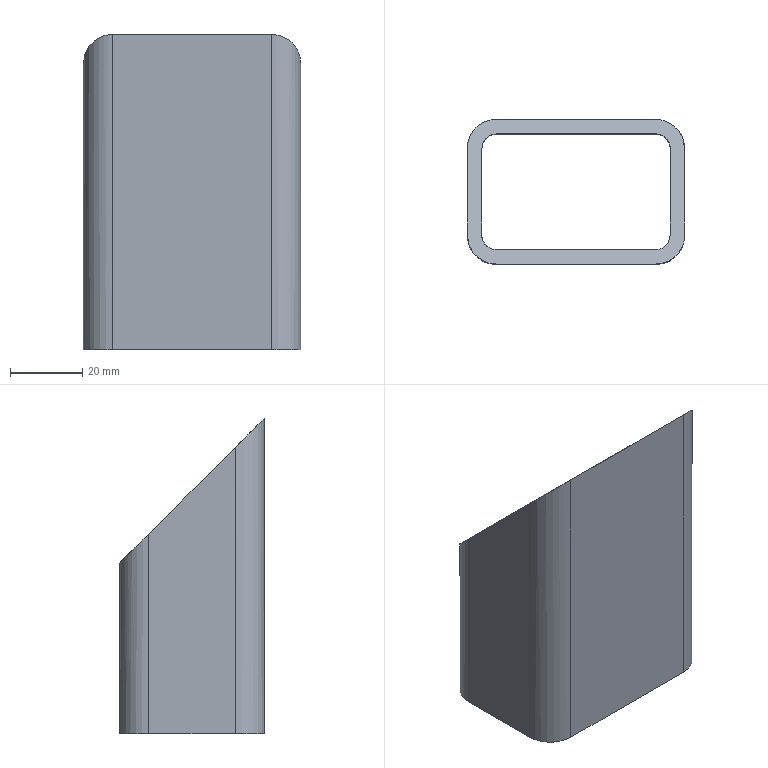Part | SolidWorks | features BaseBody 1 | 1 solid | 18 faces | box 60 x 40 x 87 mm | volume 46551 mm3 | plane 10 | cylinder 8 | commonest cylinder face diameters 8 x4 16 x4
STEP:
#1=CARTESIAN_POINT('',(22.,-20.,0.));
#2=VERTEX_POINT('',#1);
#3=CARTESIAN_POINT('',(22.,-20.,87.));
#4=VERTEX_POINT('',#3);
#5=CARTESIAN_POINT('',(22.,-20.,0.));
#6=DIRECTION('',(0.,0.,1.));
#7=VECTOR('',#6,1000.);
#8=LINE('',#5,#7);
#9=EDGE_CURVE('',#2,#4,#8,.T.);
#10=ORIENTED_EDGE('',*,*,#9,.T.);
#11=CARTESIAN_POINT('',(-22.,-20.,87.));
#12=VERTEX_POINT('',#11);
#13=CARTESIAN_POINT('',(-22.,-20.,87.));
#14=DIRECTION('',(-1.,0.,0.));
#15=VECTOR('',#14,1000.);
#16=LINE('',#13,#15);
#17=EDGE_CURVE('',#4,#12,#16,.T.);
#18=ORIENTED_EDGE('',*,*,#17,.T.);
#19=CARTESIAN_POINT('',(-22.,-20.,0.));
#20=VERTEX_POINT('',#19);
#21=CARTESIAN_POINT('',(-22.,-20.,0.));
#22=DIRECTION('',(0.,0.,-1.));
#23=VECTOR('',#22,1000.);
#24=LINE('',#21,#23);
#25=EDGE_CURVE('',#12,#20,#24,.T.);
#26=ORIENTED_EDGE('',*,*,#25,.T.);
#27=CARTESIAN_POINT('',(-22.,-20.,0.));
#28=DIRECTION('',(1.,0.,0.));
#29=VECTOR('',#28,1000.);
#30=LINE('',#27,#29);
#31=EDGE_CURVE('',#20,#2,#30,.T.);
#32=ORIENTED_EDGE('',*,*,#31,.T.);
#33=EDGE_LOOP('',(#10,#18,#26,#32));
#34=FACE_OUTER_BOUND('',#33,.T.);
#35=CARTESIAN_POINT('',(-22.,-20.,0.));
#36=DIRECTION('',(0.,-1.,0.));
#37=DIRECTION('',(0.,0.,-1.));
#38=AXIS2_PLACEMENT_3D('',#35,#36,#37);
#39=PLANE('',#38);
#40=ADVANCED_FACE('',(#34),#39,.T.);
#41=CARTESIAN_POINT('',(-26.,12.,55.));
#42=VERTEX_POINT('',#41);
#43=CARTESIAN_POINT('',(-22.,16.,51.));
#44=VERTEX_POINT('',#43);
#45=CARTESIAN_POINT('',(-26.,12.,55.));
#46=CARTESIAN_POINT('',(-26.,14.343,52.657));
#47=CARTESIAN_POINT('',(-24.343,16.,51.));
#48=CARTESIAN_POINT('',(-22.,16.,51.));
#49=(BOUNDED_CURVE()B_SPLINE_CURVE(3,(#45,#46,#47,#48),.UNSPECIFIED.,.F.,.F.)B_SPLINE_CURVE_WITH_KNOTS((4,4),(1.571,3.142),.UNSPECIFIED.)CURVE()GEOMETRIC_REPRESENTATION_ITEM()RATIONAL_B_SPLINE_CURVE((1.,0.8047,0.8047,1.))REPRESENTATION_ITEM(''));
#50=EDGE_CURVE('',#42,#44,#49,.T.);
#51=ORIENTED_EDGE('',*,*,#50,.T.);
#52=CARTESIAN_POINT('',(22.,16.,51.));
#53=VERTEX_POINT('',#52);
#54=CARTESIAN_POINT('',(-11.546,16.,51.));
#55=DIRECTION('',(1.,0.,0.));
#56=VECTOR('',#55,1000.);
#57=LINE('',#54,#56);
#58=EDGE_CURVE('',#44,#53,#57,.T.);
#59=ORIENTED_EDGE('',*,*,#58,.T.);
#60=CARTESIAN_POINT('',(26.,12.,55.));
#61=VERTEX_POINT('',#60);
#62=CARTESIAN_POINT('',(22.,16.,51.));
#63=CARTESIAN_POINT('',(24.343,16.,51.));
#64=CARTESIAN_POINT('',(26.,14.343,52.657));
#65=CARTESIAN_POINT('',(26.,12.,55.));
#66=(BOUNDED_CURVE()B_SPLINE_CURVE(3,(#62,#63,#64,#65),.UNSPECIFIED.,.F.,.F.)B_SPLINE_CURVE_WITH_KNOTS((4,4),(3.142,4.712),.UNSPECIFIED.)CURVE()GEOMETRIC_REPRESENTATION_ITEM()RATIONAL_B_SPLINE_CURVE((1.,0.8047,0.8047,1.))REPRESENTATION_ITEM(''));
#67=EDGE_CURVE('',#53,#61,#66,.T.);
#68=ORIENTED_EDGE('',*,*,#67,.T.);
#69=CARTESIAN_POINT('',(26.,-12.,79.));
#70=VERTEX_POINT('',#69);
#71=CARTESIAN_POINT('',(26.,-20.,87.));
#72=DIRECTION('',(0.,-0.7071,0.7071));
#73=VECTOR('',#72,1000.);
#74=LINE('',#71,#73);
#75=EDGE_CURVE('',#61,#70,#74,.T.);
#76=ORIENTED_EDGE('',*,*,#75,.T.);
#77=CARTESIAN_POINT('',(22.,-16.,83.));
#78=VERTEX_POINT('',#77);
#79=CARTESIAN_POINT('',(26.,-12.,79.));
#80=CARTESIAN_POINT('',(26.,-14.343,81.343));
#81=CARTESIAN_POINT('',(24.343,-16.,83.));
#82=CARTESIAN_POINT('',(22.,-16.,83.));
#83=(BOUNDED_CURVE()B_SPLINE_CURVE(3,(#79,#80,#81,#82),.UNSPECIFIED.,.F.,.F.)B_SPLINE_CURVE_WITH_KNOTS((4,4),(4.712,6.283),.UNSPECIFIED.)CURVE()GEOMETRIC_REPRESENTATION_ITEM()RATIONAL_B_SPLINE_CURVE((1.,0.8047,0.8047,1.))REPRESENTATION_ITEM(''));
#84=EDGE_CURVE('',#70,#78,#83,.T.);
#85=ORIENTED_EDGE('',*,*,#84,.T.);
#86=CARTESIAN_POINT('',(-22.,-16.,83.));
#87=VERTEX_POINT('',#86);
#88=CARTESIAN_POINT('',(-11.546,-16.,83.));
#89=DIRECTION('',(-1.,0.,0.));
#90=VECTOR('',#89,1000.);
#91=LINE('',#88,#90);
#92=EDGE_CURVE('',#78,#87,#91,.T.);
#93=ORIENTED_EDGE('',*,*,#92,.T.);
#94=CARTESIAN_POINT('',(-26.,-12.,79.));
#95=VERTEX_POINT('',#94);
#96=CARTESIAN_POINT('',(-22.,-16.,83.));
#97=CARTESIAN_POINT('',(-24.343,-16.,83.));
#98=CARTESIAN_POINT('',(-26.,-14.343,81.343));
#99=CARTESIAN_POINT('',(-26.,-12.,79.));
#100=(BOUNDED_CURVE()B_SPLINE_CURVE(3,(#96,#97,#98,#99),.UNSPECIFIED.,.F.,.F.)B_SPLINE_CURVE_WITH_KNOTS((4,4),(0.,1.571),.UNSPECIFIED.)CURVE()GEOMETRIC_REPRESENTATION_ITEM()RATIONAL_B_SPLINE_CURVE((1.,0.8047,0.8047,1.))REPRESENTATION_ITEM(''));
#101=EDGE_CURVE('',#87,#95,#100,.T.);
#102=ORIENTED_EDGE('',*,*,#101,.T.);
#103=CARTESIAN_POINT('',(-26.,-20.,87.));
#104=DIRECTION('',(0.,0.7071,-0.7071));
#105=VECTOR('',#104,1000.);
#106=LINE('',#103,#105);
#107=EDGE_CURVE('',#95,#42,#106,.T.);
#108=ORIENTED_EDGE('',*,*,#107,.T.);
#109=EDGE_LOOP('',(#51,#59,#68,#76,#85,#93,#102,#108));
#110=FACE_BOUND('',#109,.T.);
#111=CARTESIAN_POINT('',(-30.,-12.,79.));
#112=VERTEX_POINT('',#111);
#113=CARTESIAN_POINT('',(-30.,-12.,79.));
#114=CARTESIAN_POINT('',(-30.,-16.686,83.686));
#115=CARTESIAN_POINT('',(-26.686,-20.,87.));
#116=CARTESIAN_POINT('',(-22.,-20.,87.));
#117=(BOUNDED_CURVE()B_SPLINE_CURVE(3,(#113,#114,#115,#116),.UNSPECIFIED.,.F.,.F.)B_SPLINE_CURVE_WITH_KNOTS((4,4),(4.712,6.283),.UNSPECIFIED.)CURVE()GEOMETRIC_REPRESENTATION_ITEM()RATIONAL_B_SPLINE_CURVE((1.,0.8047,0.8047,1.))REPRESENTATION_ITEM(''));
#118=EDGE_CURVE('',#112,#12,#117,.T.);
#119=ORIENTED_EDGE('',*,*,#118,.T.);
#120=ORIENTED_EDGE('',*,*,#17,.F.);
#121=CARTESIAN_POINT('',(30.,-12.,79.));
#122=VERTEX_POINT('',#121);
#123=CARTESIAN_POINT('',(22.,-20.,87.));
#124=CARTESIAN_POINT('',(26.686,-20.,87.));
#125=CARTESIAN_POINT('',(30.,-16.686,83.686));
#126=CARTESIAN_POINT('',(30.,-12.,79.));
#127=(BOUNDED_CURVE()B_SPLINE_CURVE(3,(#123,#124,#125,#126),.UNSPECIFIED.,.F.,.F.)B_SPLINE_CURVE_WITH_KNOTS((4,4),(0.,1.571),.UNSPECIFIED.)CURVE()GEOMETRIC_REPRESENTATION_ITEM()RATIONAL_B_SPLINE_CURVE((1.,0.8047,0.8047,1.))REPRESENTATION_ITEM(''));
#128=EDGE_CURVE('',#4,#122,#127,.T.);
#129=ORIENTED_EDGE('',*,*,#128,.T.);
#130=CARTESIAN_POINT('',(30.,12.,55.));
#131=VERTEX_POINT('',#130);
#132=CARTESIAN_POINT('',(30.,-20.,87.));
#133=DIRECTION('',(0.,0.7071,-0.7071));
#134=VECTOR('',#133,1000.);
#135=LINE('',#132,#134);
#136=EDGE_CURVE('',#122,#131,#135,.T.);
#137=ORIENTED_EDGE('',*,*,#136,.T.);
#138=CARTESIAN_POINT('',(22.,20.,47.));
#139=VERTEX_POINT('',#138);
#140=CARTESIAN_POINT('',(30.,12.,55.));
#141=CARTESIAN_POINT('',(30.,16.686,50.314));
#142=CARTESIAN_POINT('',(26.686,20.,47.));
#143=CARTESIAN_POINT('',(22.,20.,47.));
#144=(BOUNDED_CURVE()B_SPLINE_CURVE(3,(#140,#141,#142,#143),.UNSPECIFIED.,.F.,.F.)B_SPLINE_CURVE_WITH_KNOTS((4,4),(1.571,3.142),.UNSPECIFIED.)CURVE()GEOMETRIC_REPRESENTATION_ITEM()RATIONAL_B_SPLINE_CURVE((1.,0.8047,0.8047,1.))REPRESENTATION_ITEM(''));
#145=EDGE_CURVE('',#131,#139,#144,.T.);
#146=ORIENTED_EDGE('',*,*,#145,.T.);
#147=CARTESIAN_POINT('',(-22.,20.,47.));
#148=VERTEX_POINT('',#147);
#149=CARTESIAN_POINT('',(-11.546,20.,47.));
#150=DIRECTION('',(-1.,0.,0.));
#151=VECTOR('',#150,1000.);
#152=LINE('',#149,#151);
#153=EDGE_CURVE('',#139,#148,#152,.T.);
#154=ORIENTED_EDGE('',*,*,#153,.T.);
#155=CARTESIAN_POINT('',(-30.,12.,55.));
#156=VERTEX_POINT('',#155);
#157=CARTESIAN_POINT('',(-22.,20.,47.));
#158=CARTESIAN_POINT('',(-26.686,20.,47.));
#159=CARTESIAN_POINT('',(-30.,16.686,50.314));
#160=CARTESIAN_POINT('',(-30.,12.,55.));
#161=(BOUNDED_CURVE()B_SPLINE_CURVE(3,(#157,#158,#159,#160),.UNSPECIFIED.,.F.,.T.)B_SPLINE_CURVE_WITH_KNOTS((4,4),(3.142,4.712),.UNSPECIFIED.)CURVE()GEOMETRIC_REPRESENTATION_ITEM()RATIONAL_B_SPLINE_CURVE((1.,0.8047,0.8047,1.))REPRESENTATION_ITEM(''));
#162=EDGE_CURVE('',#148,#156,#161,.T.);
#163=ORIENTED_EDGE('',*,*,#162,.T.);
#164=CARTESIAN_POINT('',(-30.,-20.,87.));
#165=DIRECTION('',(0.,-0.7071,0.7071));
#166=VECTOR('',#165,1000.);
#167=LINE('',#164,#166);
#168=EDGE_CURVE('',#156,#112,#167,.T.);
#169=ORIENTED_EDGE('',*,*,#168,.T.);
#170=EDGE_LOOP('',(#119,#120,#129,#137,#146,#154,#163,#169));
#171=FACE_OUTER_BOUND('',#170,.T.);
#172=CARTESIAN_POINT('',(-11.546,-20.,87.));
#173=DIRECTION('',(0.,0.7071,0.7071));
#174=DIRECTION('',(0.,-0.7071,0.7071));
#175=AXIS2_PLACEMENT_3D('',#172,#173,#174);
#176=PLANE('',#175);
#177=ADVANCED_FACE('',(#110,#171),#176,.T.);
#178=CARTESIAN_POINT('',(30.,-12.,0.));
#179=VERTEX_POINT('',#178);
#180=CARTESIAN_POINT('',(30.,-12.,0.));
#181=DIRECTION('',(0.,0.,1.));
#182=VECTOR('',#181,1000.);
#183=LINE('',#180,#182);
#184=EDGE_CURVE('',#179,#122,#183,.T.);
#185=ORIENTED_EDGE('',*,*,#184,.T.);
#186=ORIENTED_EDGE('',*,*,#128,.F.);
#187=ORIENTED_EDGE('',*,*,#9,.F.);
#188=CARTESIAN_POINT('',(22.,-12.,0.));
#189=DIRECTION('',(0.,0.,1.));
#190=DIRECTION('',(1.,0.,0.));
#191=AXIS2_PLACEMENT_3D('',#188,#189,#190);
#192=CIRCLE('',#191,8.);
#193=EDGE_CURVE('',#2,#179,#192,.T.);
#194=ORIENTED_EDGE('',*,*,#193,.T.);
#195=EDGE_LOOP('',(#185,#186,#187,#194));
#196=FACE_OUTER_BOUND('',#195,.T.);
#197=CARTESIAN_POINT('',(22.,-12.,0.));
#198=DIRECTION('',(0.,0.,1.));
#199=DIRECTION('',(1.,0.,0.));
#200=AXIS2_PLACEMENT_3D('',#197,#198,#199);
#201=CYLINDRICAL_SURFACE('',#200,8.);
#202=ADVANCED_FACE('',(#196),#201,.T.);
#203=CARTESIAN_POINT('',(-26.,-12.,0.));
#204=VERTEX_POINT('',#203);
#205=CARTESIAN_POINT('',(-26.,12.,0.));
#206=VERTEX_POINT('',#205);
#207=CARTESIAN_POINT('',(-26.,0.,0.));
#208=DIRECTION('',(0.,1.,0.));
#209=VECTOR('',#208,1000.);
#210=LINE('',#207,#209);
#211=EDGE_CURVE('',#204,#206,#210,.T.);
#212=ORIENTED_EDGE('',*,*,#211,.F.);
#213=CARTESIAN_POINT('',(-22.,-16.,0.));
#214=VERTEX_POINT('',#213);
#215=CARTESIAN_POINT('',(-22.,-12.,0.));
#216=DIRECTION('',(0.,0.,-1.));
#217=DIRECTION('',(1.,0.,0.));
#218=AXIS2_PLACEMENT_3D('',#215,#216,#217);
#219=CIRCLE('',#218,4.);
#220=EDGE_CURVE('',#214,#204,#219,.T.);
#221=ORIENTED_EDGE('',*,*,#220,.F.);
#222=CARTESIAN_POINT('',(22.,-16.,0.));
#223=VERTEX_POINT('',#222);
#224=CARTESIAN_POINT('',(0.,-16.,0.));
#225=DIRECTION('',(-1.,0.,0.));
#226=VECTOR('',#225,1000.);
#227=LINE('',#224,#226);
#228=EDGE_CURVE('',#223,#214,#227,.T.);
#229=ORIENTED_EDGE('',*,*,#228,.F.);
#230=CARTESIAN_POINT('',(26.,-12.,0.));
#231=VERTEX_POINT('',#230);
#232=CARTESIAN_POINT('',(22.,-12.,0.));
#233=DIRECTION('',(0.,0.,-1.));
#234=DIRECTION('',(1.,0.,0.));
#235=AXIS2_PLACEMENT_3D('',#232,#233,#234);
#236=CIRCLE('',#235,4.);
#237=EDGE_CURVE('',#231,#223,#236,.T.);
#238=ORIENTED_EDGE('',*,*,#237,.F.);
#239=CARTESIAN_POINT('',(26.,12.,0.));
#240=VERTEX_POINT('',#239);
#241=CARTESIAN_POINT('',(26.,0.,0.));
#242=DIRECTION('',(0.,-1.,0.));
#243=VECTOR('',#242,1000.);
#244=LINE('',#241,#243);
#245=EDGE_CURVE('',#240,#231,#244,.T.);
#246=ORIENTED_EDGE('',*,*,#245,.F.);
#247=CARTESIAN_POINT('',(22.,16.,0.));
#248=VERTEX_POINT('',#247);
#249=CARTESIAN_POINT('',(22.,12.,0.));
#250=DIRECTION('',(0.,0.,-1.));
#251=DIRECTION('',(1.,0.,0.));
#252=AXIS2_PLACEMENT_3D('',#249,#250,#251);
#253=CIRCLE('',#252,4.);
#254=EDGE_CURVE('',#248,#240,#253,.T.);
#255=ORIENTED_EDGE('',*,*,#254,.F.);
#256=CARTESIAN_POINT('',(-22.,16.,0.));
#257=VERTEX_POINT('',#256);
#258=CARTESIAN_POINT('',(0.,16.,0.));
#259=DIRECTION('',(1.,0.,0.));
#260=VECTOR('',#259,1000.);
#261=LINE('',#258,#260);
#262=EDGE_CURVE('',#257,#248,#261,.T.);
#263=ORIENTED_EDGE('',*,*,#262,.F.);
#264=CARTESIAN_POINT('',(-22.,12.,0.));
#265=DIRECTION('',(0.,0.,-1.));
#266=DIRECTION('',(1.,0.,0.));
#267=AXIS2_PLACEMENT_3D('',#264,#265,#266);
#268=CIRCLE('',#267,4.);
#269=EDGE_CURVE('',#206,#257,#268,.T.);
#270=ORIENTED_EDGE('',*,*,#269,.F.);
#271=EDGE_LOOP('',(#212,#221,#229,#238,#246,#255,#263,#270));
#272=FACE_BOUND('',#271,.T.);
#273=CARTESIAN_POINT('',(30.,12.,0.));
#274=VERTEX_POINT('',#273);
#275=CARTESIAN_POINT('',(22.,20.,0.));
#276=VERTEX_POINT('',#275);
#277=CARTESIAN_POINT('',(22.,12.,0.));
#278=DIRECTION('',(0.,0.,1.));
#279=DIRECTION('',(1.,0.,0.));
#280=AXIS2_PLACEMENT_3D('',#277,#278,#279);
#281=CIRCLE('',#280,8.);
#282=EDGE_CURVE('',#274,#276,#281,.T.);
#283=ORIENTED_EDGE('',*,*,#282,.F.);
#284=CARTESIAN_POINT('',(30.,0.,0.));
#285=DIRECTION('',(0.,1.,0.));
#286=VECTOR('',#285,1000.);
#287=LINE('',#284,#286);
#288=EDGE_CURVE('',#179,#274,#287,.T.);
#289=ORIENTED_EDGE('',*,*,#288,.F.);
#290=ORIENTED_EDGE('',*,*,#193,.F.);
#291=ORIENTED_EDGE('',*,*,#31,.F.);
#292=CARTESIAN_POINT('',(-30.,-12.,0.));
#293=VERTEX_POINT('',#292);
#294=CARTESIAN_POINT('',(-22.,-12.,0.));
#295=DIRECTION('',(0.,0.,1.));
#296=DIRECTION('',(1.,0.,0.));
#297=AXIS2_PLACEMENT_3D('',#294,#295,#296);
#298=CIRCLE('',#297,8.);
#299=EDGE_CURVE('',#293,#20,#298,.T.);
#300=ORIENTED_EDGE('',*,*,#299,.F.);
#301=CARTESIAN_POINT('',(-30.,12.,0.));
#302=VERTEX_POINT('',#301);
#303=CARTESIAN_POINT('',(-30.,0.,0.));
#304=DIRECTION('',(0.,-1.,0.));
#305=VECTOR('',#304,1000.);
#306=LINE('',#303,#305);
#307=EDGE_CURVE('',#302,#293,#306,.T.);
#308=ORIENTED_EDGE('',*,*,#307,.F.);
#309=CARTESIAN_POINT('',(-22.,20.,0.));
#310=VERTEX_POINT('',#309);
#311=CARTESIAN_POINT('',(-22.,12.,0.));
#312=DIRECTION('',(0.,0.,1.));
#313=DIRECTION('',(1.,0.,0.));
#314=AXIS2_PLACEMENT_3D('',#311,#312,#313);
#315=CIRCLE('',#314,8.);
#316=EDGE_CURVE('',#310,#302,#315,.T.);
#317=ORIENTED_EDGE('',*,*,#316,.F.);
#318=CARTESIAN_POINT('',(0.,20.,0.));
#319=DIRECTION('',(-1.,0.,0.));
#320=VECTOR('',#319,1000.);
#321=LINE('',#318,#320);
#322=EDGE_CURVE('',#276,#310,#321,.T.);
#323=ORIENTED_EDGE('',*,*,#322,.F.);
#324=EDGE_LOOP('',(#283,#289,#290,#291,#300,#308,#317,#323));
#325=FACE_OUTER_BOUND('',#324,.T.);
#326=CARTESIAN_POINT('',(0.,0.,0.));
#327=DIRECTION('',(0.,0.,1.));
#328=DIRECTION('',(1.,0.,0.));
#329=AXIS2_PLACEMENT_3D('',#326,#327,#328);
#330=PLANE('',#329);
#331=ADVANCED_FACE('',(#272,#325),#330,.F.);
#332=ORIENTED_EDGE('',*,*,#25,.F.);
#333=ORIENTED_EDGE('',*,*,#118,.F.);
#334=CARTESIAN_POINT('',(-30.,-12.,0.));
#335=DIRECTION('',(0.,0.,-1.));
#336=VECTOR('',#335,1000.);
#337=LINE('',#334,#336);
#338=EDGE_CURVE('',#112,#293,#337,.T.);
#339=ORIENTED_EDGE('',*,*,#338,.T.);
#340=ORIENTED_EDGE('',*,*,#299,.T.);
#341=EDGE_LOOP('',(#332,#333,#339,#340));
#342=FACE_OUTER_BOUND('',#341,.T.);
#343=CARTESIAN_POINT('',(-22.,-12.,0.));
#344=DIRECTION('',(0.,0.,1.));
#345=DIRECTION('',(1.,0.,0.));
#346=AXIS2_PLACEMENT_3D('',#343,#344,#345);
#347=CYLINDRICAL_SURFACE('',#346,8.);
#348=ADVANCED_FACE('',(#342),#347,.T.);
#349=CARTESIAN_POINT('',(22.,16.,0.));
#350=DIRECTION('',(0.,0.,1.));
#351=VECTOR('',#350,1000.);
#352=LINE('',#349,#351);
#353=EDGE_CURVE('',#248,#53,#352,.T.);
#354=ORIENTED_EDGE('',*,*,#353,.T.);
#355=ORIENTED_EDGE('',*,*,#58,.F.);
#356=CARTESIAN_POINT('',(-22.,16.,0.));
#357=DIRECTION('',(0.,0.,-1.));
#358=VECTOR('',#357,1000.);
#359=LINE('',#356,#358);
#360=EDGE_CURVE('',#44,#257,#359,.T.);
#361=ORIENTED_EDGE('',*,*,#360,.T.);
#362=ORIENTED_EDGE('',*,*,#262,.T.);
#363=EDGE_LOOP('',(#354,#355,#361,#362));
#364=FACE_OUTER_BOUND('',#363,.T.);
#365=CARTESIAN_POINT('',(-22.,16.,0.));
#366=DIRECTION('',(0.,-1.,0.));
#367=DIRECTION('',(0.,0.,-1.));
#368=AXIS2_PLACEMENT_3D('',#365,#366,#367);
#369=PLANE('',#368);
#370=ADVANCED_FACE('',(#364),#369,.T.);
#371=ORIENTED_EDGE('',*,*,#269,.T.);
#372=ORIENTED_EDGE('',*,*,#360,.F.);
#373=ORIENTED_EDGE('',*,*,#50,.F.);
#374=CARTESIAN_POINT('',(-26.,12.,0.));
#375=DIRECTION('',(0.,0.,1.));
#376=VECTOR('',#375,1000.);
#377=LINE('',#374,#376);
#378=EDGE_CURVE('',#206,#42,#377,.T.);
#379=ORIENTED_EDGE('',*,*,#378,.F.);
#380=EDGE_LOOP('',(#371,#372,#373,#379));
#381=FACE_OUTER_BOUND('',#380,.T.);
#382=CARTESIAN_POINT('',(-22.,12.,0.));
#383=DIRECTION('',(0.,0.,1.));
#384=DIRECTION('',(1.,0.,0.));
#385=AXIS2_PLACEMENT_3D('',#382,#383,#384);
#386=CYLINDRICAL_SURFACE('',#385,4.);
#387=ADVANCED_FACE('',(#381),#386,.F.);
#388=ORIENTED_EDGE('',*,*,#378,.T.);
#389=ORIENTED_EDGE('',*,*,#107,.F.);
#390=CARTESIAN_POINT('',(-26.,-12.,0.));
#391=DIRECTION('',(0.,0.,-1.));
#392=VECTOR('',#391,1000.);
#393=LINE('',#390,#392);
#394=EDGE_CURVE('',#95,#204,#393,.T.);
#395=ORIENTED_EDGE('',*,*,#394,.T.);
#396=ORIENTED_EDGE('',*,*,#211,.T.);
#397=EDGE_LOOP('',(#388,#389,#395,#396));
#398=FACE_OUTER_BOUND('',#397,.T.);
#399=CARTESIAN_POINT('',(-26.,-12.,0.));
#400=DIRECTION('',(1.,0.,0.));
#401=DIRECTION('',(0.,0.,-1.));
#402=AXIS2_PLACEMENT_3D('',#399,#400,#401);
#403=PLANE('',#402);
#404=ADVANCED_FACE('',(#398),#403,.T.);
#405=ORIENTED_EDGE('',*,*,#220,.T.);
#406=ORIENTED_EDGE('',*,*,#394,.F.);
#407=ORIENTED_EDGE('',*,*,#101,.F.);
#408=CARTESIAN_POINT('',(-22.,-16.,0.));
#409=DIRECTION('',(0.,0.,1.));
#410=VECTOR('',#409,1000.);
#411=LINE('',#408,#410);
#412=EDGE_CURVE('',#214,#87,#411,.T.);
#413=ORIENTED_EDGE('',*,*,#412,.F.);
#414=EDGE_LOOP('',(#405,#406,#407,#413));
#415=FACE_OUTER_BOUND('',#414,.T.);
#416=CARTESIAN_POINT('',(-22.,-12.,0.));
#417=DIRECTION('',(0.,0.,1.));
#418=DIRECTION('',(1.,0.,0.));
#419=AXIS2_PLACEMENT_3D('',#416,#417,#418);
#420=CYLINDRICAL_SURFACE('',#419,4.);
#421=ADVANCED_FACE('',(#415),#420,.F.);
#422=ORIENTED_EDGE('',*,*,#412,.T.);
#423=ORIENTED_EDGE('',*,*,#92,.F.);
#424=CARTESIAN_POINT('',(22.,-16.,0.));
#425=DIRECTION('',(0.,0.,-1.));
#426=VECTOR('',#425,1000.);
#427=LINE('',#424,#426);
#428=EDGE_CURVE('',#78,#223,#427,.T.);
#429=ORIENTED_EDGE('',*,*,#428,.T.);
#430=ORIENTED_EDGE('',*,*,#228,.T.);
#431=EDGE_LOOP('',(#422,#423,#429,#430));
#432=FACE_OUTER_BOUND('',#431,.T.);
#433=CARTESIAN_POINT('',(22.,-16.,0.));
#434=DIRECTION('',(0.,1.,0.));
#435=DIRECTION('',(0.,0.,1.));
#436=AXIS2_PLACEMENT_3D('',#433,#434,#435);
#437=PLANE('',#436);
#438=ADVANCED_FACE('',(#432),#437,.T.);
#439=ORIENTED_EDGE('',*,*,#237,.T.);
#440=ORIENTED_EDGE('',*,*,#428,.F.);
#441=ORIENTED_EDGE('',*,*,#84,.F.);
#442=CARTESIAN_POINT('',(26.,-12.,0.));
#443=DIRECTION('',(0.,0.,1.));
#444=VECTOR('',#443,1000.);
#445=LINE('',#442,#444);
#446=EDGE_CURVE('',#231,#70,#445,.T.);
#447=ORIENTED_EDGE('',*,*,#446,.F.);
#448=EDGE_LOOP('',(#439,#440,#441,#447));
#449=FACE_OUTER_BOUND('',#448,.T.);
#450=CARTESIAN_POINT('',(22.,-12.,0.));
#451=DIRECTION('',(0.,0.,1.));
#452=DIRECTION('',(1.,0.,0.));
#453=AXIS2_PLACEMENT_3D('',#450,#451,#452);
#454=CYLINDRICAL_SURFACE('',#453,4.);
#455=ADVANCED_FACE('',(#449),#454,.F.);
#456=ORIENTED_EDGE('',*,*,#446,.T.);
#457=ORIENTED_EDGE('',*,*,#75,.F.);
#458=CARTESIAN_POINT('',(26.,12.,0.));
#459=DIRECTION('',(0.,0.,-1.));
#460=VECTOR('',#459,1000.);
#461=LINE('',#458,#460);
#462=EDGE_CURVE('',#61,#240,#461,.T.);
#463=ORIENTED_EDGE('',*,*,#462,.T.);
#464=ORIENTED_EDGE('',*,*,#245,.T.);
#465=EDGE_LOOP('',(#456,#457,#463,#464));
#466=FACE_OUTER_BOUND('',#465,.T.);
#467=CARTESIAN_POINT('',(26.,12.,0.));
#468=DIRECTION('',(-1.,0.,0.));
#469=DIRECTION('',(0.,0.,1.));
#470=AXIS2_PLACEMENT_3D('',#467,#468,#469);
#471=PLANE('',#470);
#472=ADVANCED_FACE('',(#466),#471,.T.);
#473=ORIENTED_EDGE('',*,*,#254,.T.);
#474=ORIENTED_EDGE('',*,*,#462,.F.);
#475=ORIENTED_EDGE('',*,*,#67,.F.);
#476=ORIENTED_EDGE('',*,*,#353,.F.);
#477=EDGE_LOOP('',(#473,#474,#475,#476));
#478=FACE_OUTER_BOUND('',#477,.T.);
#479=CARTESIAN_POINT('',(22.,12.,0.));
#480=DIRECTION('',(0.,0.,1.));
#481=DIRECTION('',(1.,0.,0.));
#482=AXIS2_PLACEMENT_3D('',#479,#480,#481);
#483=CYLINDRICAL_SURFACE('',#482,4.);
#484=ADVANCED_FACE('',(#478),#483,.F.);
#485=ORIENTED_EDGE('',*,*,#338,.F.);
#486=ORIENTED_EDGE('',*,*,#168,.F.);
#487=CARTESIAN_POINT('',(-30.,12.,0.));
#488=DIRECTION('',(0.,0.,-1.));
#489=VECTOR('',#488,1000.);
#490=LINE('',#487,#489);
#491=EDGE_CURVE('',#156,#302,#490,.T.);
#492=ORIENTED_EDGE('',*,*,#491,.T.);
#493=ORIENTED_EDGE('',*,*,#307,.T.);
#494=EDGE_LOOP('',(#485,#486,#492,#493));
#495=FACE_OUTER_BOUND('',#494,.T.);
#496=CARTESIAN_POINT('',(-30.,12.,0.));
#497=DIRECTION('',(-1.,0.,0.));
#498=DIRECTION('',(0.,0.,1.));
#499=AXIS2_PLACEMENT_3D('',#496,#497,#498);
#500=PLANE('',#499);
#501=ADVANCED_FACE('',(#495),#500,.T.);
#502=ORIENTED_EDGE('',*,*,#491,.F.);
#503=ORIENTED_EDGE('',*,*,#162,.F.);
#504=CARTESIAN_POINT('',(-22.,20.,0.));
#505=DIRECTION('',(0.,0.,-1.));
#506=VECTOR('',#505,1000.);
#507=LINE('',#504,#506);
#508=EDGE_CURVE('',#148,#310,#507,.T.);
#509=ORIENTED_EDGE('',*,*,#508,.T.);
#510=ORIENTED_EDGE('',*,*,#316,.T.);
#511=EDGE_LOOP('',(#502,#503,#509,#510));
#512=FACE_OUTER_BOUND('',#511,.T.);
#513=CARTESIAN_POINT('',(-22.,12.,0.));
#514=DIRECTION('',(0.,0.,1.));
#515=DIRECTION('',(1.,0.,0.));
#516=AXIS2_PLACEMENT_3D('',#513,#514,#515);
#517=CYLINDRICAL_SURFACE('',#516,8.);
#518=ADVANCED_FACE('',(#512),#517,.T.);
#519=ORIENTED_EDGE('',*,*,#508,.F.);
#520=ORIENTED_EDGE('',*,*,#153,.F.);
#521=CARTESIAN_POINT('',(22.,20.,0.));
#522=DIRECTION('',(0.,0.,-1.));
#523=VECTOR('',#522,1000.);
#524=LINE('',#521,#523);
#525=EDGE_CURVE('',#139,#276,#524,.T.);
#526=ORIENTED_EDGE('',*,*,#525,.T.);
#527=ORIENTED_EDGE('',*,*,#322,.T.);
#528=EDGE_LOOP('',(#519,#520,#526,#527));
#529=FACE_OUTER_BOUND('',#528,.T.);
#530=CARTESIAN_POINT('',(22.,20.,0.));
#531=DIRECTION('',(0.,1.,0.));
#532=DIRECTION('',(0.,0.,1.));
#533=AXIS2_PLACEMENT_3D('',#530,#531,#532);
#534=PLANE('',#533);
#535=ADVANCED_FACE('',(#529),#534,.T.);
#536=ORIENTED_EDGE('',*,*,#525,.F.);
#537=ORIENTED_EDGE('',*,*,#145,.F.);
#538=CARTESIAN_POINT('',(30.,12.,0.));
#539=DIRECTION('',(0.,0.,-1.));
#540=VECTOR('',#539,1000.);
#541=LINE('',#538,#540);
#542=EDGE_CURVE('',#131,#274,#541,.T.);
#543=ORIENTED_EDGE('',*,*,#542,.T.);
#544=ORIENTED_EDGE('',*,*,#282,.T.);
#545=EDGE_LOOP('',(#536,#537,#543,#544));
#546=FACE_OUTER_BOUND('',#545,.T.);
#547=CARTESIAN_POINT('',(22.,12.,0.));
#548=DIRECTION('',(0.,0.,1.));
#549=DIRECTION('',(1.,0.,0.));
#550=AXIS2_PLACEMENT_3D('',#547,#548,#549);
#551=CYLINDRICAL_SURFACE('',#550,8.);
#552=ADVANCED_FACE('',(#546),#551,.T.);
#553=ORIENTED_EDGE('',*,*,#542,.F.);
#554=ORIENTED_EDGE('',*,*,#136,.F.);
#555=ORIENTED_EDGE('',*,*,#184,.F.);
#556=ORIENTED_EDGE('',*,*,#288,.T.);
#557=EDGE_LOOP('',(#553,#554,#555,#556));
#558=FACE_OUTER_BOUND('',#557,.T.);
#559=CARTESIAN_POINT('',(30.,-12.,0.));
#560=DIRECTION('',(1.,0.,0.));
#561=DIRECTION('',(0.,0.,-1.));
#562=AXIS2_PLACEMENT_3D('',#559,#560,#561);
#563=PLANE('',#562);
#564=ADVANCED_FACE('',(#558),#563,.T.);
#565=CLOSED_SHELL('',(#40,#177,#202,#331,#348,#370,#387,#404,#421,#438,#455,#472,#484,#501,#518,#535,#552,#564));
#566=MANIFOLD_SOLID_BREP('',#565);
#567=CARTESIAN_POINT('',(0.,0.,0.));
#568=DIRECTION('',(0.,0.,1.));
#569=DIRECTION('',(1.,0.,0.));
#570=AXIS2_PLACEMENT_3D('',#567,#568,#569);
#571=(LENGTH_UNIT()NAMED_UNIT(*)SI_UNIT(.MILLI.,.METRE.));
#572=UNCERTAINTY_MEASURE_WITH_UNIT(LENGTH_MEASURE(0.00001),#571,'','');
#573=(NAMED_UNIT(*)PLANE_ANGLE_UNIT()SI_UNIT($,.RADIAN.));
#574=(NAMED_UNIT(*)SI_UNIT($,.STERADIAN.)SOLID_ANGLE_UNIT());
#575=(GEOMETRIC_REPRESENTATION_CONTEXT(3)GLOBAL_UNCERTAINTY_ASSIGNED_CONTEXT((#572))GLOBAL_UNIT_ASSIGNED_CONTEXT((#571,#573,#574))REPRESENTATION_CONTEXT('',''));
#576=ADVANCED_BREP_SHAPE_REPRESENTATION('',(#566,#570),#575);